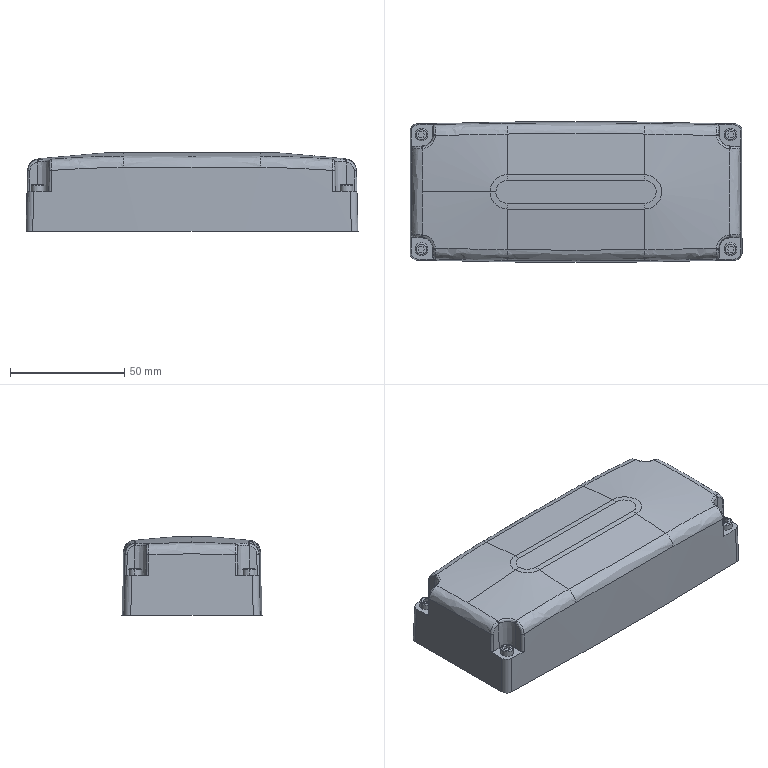Part | SolidWorks | 6 solids | 195 faces | box 145.001 x 61.5 x 34.5 mm | volume 436021 mm3 | plane 80 | spline 58 | cone 33 | cylinder 24 | commonest cylinder face diameters 3.195 x8 5.5 x8 2 x4 55.6 x2 60 x2